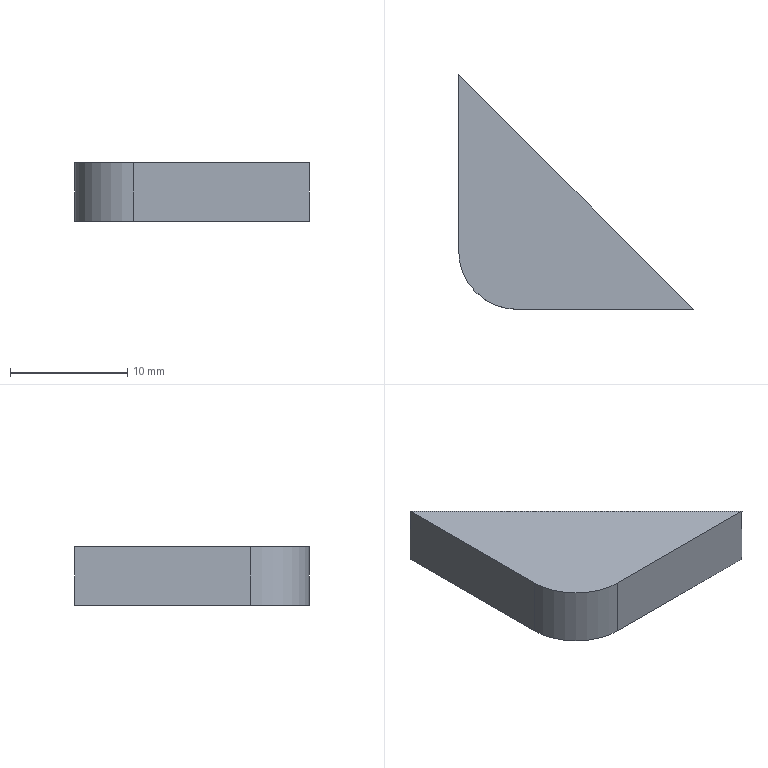Part | STEP file | Part8_5 | 1 solid | 6 faces | box 20 x 20 x 5 mm | volume 973.175 mm3 | plane 5 | cylinder 1 | commonest cylinder face diameters 10 x1
STEP:
#1=CARTESIAN_POINT('',(0.,0.,0.));
#2=DIRECTION('',(0.,0.,1.));
#3=DIRECTION('',(1.,0.,0.));
#4=AXIS2_PLACEMENT_3D('',#1,#2,#3);
#5=CARTESIAN_POINT('',(150.,24.941,-720.));
#6=VERTEX_POINT('',#5);
#7=CARTESIAN_POINT('',(130.,44.941,-720.));
#8=VERTEX_POINT('',#7);
#9=CARTESIAN_POINT('',(130.,44.941,-720.));
#10=DIRECTION('',(-0.7071,0.7071,0.));
#11=VECTOR('',#10,1.);
#12=LINE('',#9,#11);
#13=CARTESIAN_POINT('',(0.,0.,-720.));
#14=DIRECTION('',(0.,0.,-1.));
#15=DIRECTION('',(-1.,0.,0.));
#16=AXIS2_PLACEMENT_3D('',#13,#14,#15);
#17=PLANE('',#16);
#18=CARTESIAN_POINT('',(-130.,44.941));
#19=DIRECTION('',(0.7071,0.7071));
#20=VECTOR('',#19,1.);
#21=LINE('',#18,#20);
#22=(GEOMETRIC_REPRESENTATION_CONTEXT(2)PARAMETRIC_REPRESENTATION_CONTEXT()REPRESENTATION_CONTEXT('',''));
#23=DEFINITIONAL_REPRESENTATION('',(#21),#22);
#24=PCURVE('',#17,#23);
#25=CARTESIAN_POINT('',(130.,44.941,-685.));
#26=DIRECTION('',(0.7071,0.7071,0.));
#27=DIRECTION('',(-0.7071,0.7071,0.));
#28=AXIS2_PLACEMENT_3D('',#25,#26,#27);
#29=PLANE('',#28);
#30=CARTESIAN_POINT('',(0.,-35.));
#31=DIRECTION('',(1.,0.));
#32=VECTOR('',#31,1.);
#33=LINE('',#30,#32);
#34=(GEOMETRIC_REPRESENTATION_CONTEXT(2)PARAMETRIC_REPRESENTATION_CONTEXT()REPRESENTATION_CONTEXT('',''));
#35=DEFINITIONAL_REPRESENTATION('',(#33),#34);
#36=PCURVE('',#29,#35);
#37=SURFACE_CURVE('',#12,(#24,#36),.PCURVE_S1.);
#38=EDGE_CURVE('',#6,#8,#37,.T.);
#39=ORIENTED_EDGE('',*,*,#38,.F.);
#40=CARTESIAN_POINT('',(135.,24.941,-720.));
#41=VERTEX_POINT('',#40);
#42=CARTESIAN_POINT('',(135.,24.941,-720.));
#43=DIRECTION('',(-1.,0.,0.));
#44=VECTOR('',#43,1.);
#45=LINE('',#42,#44);
#46=CARTESIAN_POINT('',(-135.,24.941));
#47=DIRECTION('',(1.,0.));
#48=VECTOR('',#47,1.);
#49=LINE('',#46,#48);
#50=(GEOMETRIC_REPRESENTATION_CONTEXT(2)PARAMETRIC_REPRESENTATION_CONTEXT()REPRESENTATION_CONTEXT('',''));
#51=DEFINITIONAL_REPRESENTATION('',(#49),#50);
#52=PCURVE('',#17,#51);
#53=CARTESIAN_POINT('',(135.,24.941,-685.));
#54=DIRECTION('',(0.,1.,0.));
#55=DIRECTION('',(-1.,0.,0.));
#56=AXIS2_PLACEMENT_3D('',#53,#54,#55);
#57=PLANE('',#56);
#58=CARTESIAN_POINT('',(0.,-35.));
#59=DIRECTION('',(1.,0.));
#60=VECTOR('',#59,1.);
#61=LINE('',#58,#60);
#62=(GEOMETRIC_REPRESENTATION_CONTEXT(2)PARAMETRIC_REPRESENTATION_CONTEXT()REPRESENTATION_CONTEXT('',''));
#63=DEFINITIONAL_REPRESENTATION('',(#61),#62);
#64=PCURVE('',#57,#63);
#65=SURFACE_CURVE('',#45,(#52,#64),.PCURVE_S1.);
#66=EDGE_CURVE('',#6,#41,#65,.T.);
#67=ORIENTED_EDGE('',*,*,#66,.T.);
#68=CARTESIAN_POINT('',(130.,29.941,-720.));
#69=VERTEX_POINT('',#68);
#70=CARTESIAN_POINT('',(135.,29.941,-720.));
#71=DIRECTION('',(0.,0.,1.));
#72=DIRECTION('',(-1.,0.,0.));
#73=AXIS2_PLACEMENT_3D('',#70,#71,#72);
#74=CIRCLE('',#73,5.);
#75=CARTESIAN_POINT('',(-130.,29.941));
#76=CARTESIAN_POINT('',(-130.,21.281));
#77=CARTESIAN_POINT('',(-137.5,25.611));
#78=CARTESIAN_POINT('',(-145.,29.941));
#79=CARTESIAN_POINT('',(-137.5,34.271));
#80=CARTESIAN_POINT('',(-130.,38.602));
#81=CARTESIAN_POINT('',(-130.,29.941));
#82=(BOUNDED_CURVE()B_SPLINE_CURVE(2,(#75,#76,#77,#78,#79,#80,#81),.UNSPECIFIED.,.T.,.F.)B_SPLINE_CURVE_WITH_KNOTS((1,2,2,2,2,1),(-2.094,0.,2.094,4.189,6.283,8.378),.UNSPECIFIED.)CURVE()GEOMETRIC_REPRESENTATION_ITEM()RATIONAL_B_SPLINE_CURVE((1.,0.5,1.,0.5,1.,0.5,1.))REPRESENTATION_ITEM(''));
#83=(GEOMETRIC_REPRESENTATION_CONTEXT(2)PARAMETRIC_REPRESENTATION_CONTEXT()REPRESENTATION_CONTEXT('',''));
#84=DEFINITIONAL_REPRESENTATION('',(#82),#83);
#85=PCURVE('',#17,#84);
#86=CARTESIAN_POINT('',(135.,29.941,-717.5));
#87=DIRECTION('',(0.,0.,-1.));
#88=DIRECTION('',(-1.,0.,0.));
#89=AXIS2_PLACEMENT_3D('',#86,#87,#88);
#90=CYLINDRICAL_SURFACE('',#89,5.);
#91=CARTESIAN_POINT('',(6.283,2.5));
#92=DIRECTION('',(-1.,0.));
#93=VECTOR('',#92,1.);
#94=LINE('',#91,#93);
#95=(GEOMETRIC_REPRESENTATION_CONTEXT(2)PARAMETRIC_REPRESENTATION_CONTEXT()REPRESENTATION_CONTEXT('',''));
#96=DEFINITIONAL_REPRESENTATION('',(#94),#95);
#97=PCURVE('',#90,#96);
#98=SURFACE_CURVE('',#74,(#85,#97),.PCURVE_S1.);
#99=EDGE_CURVE('',#69,#41,#98,.T.);
#100=ORIENTED_EDGE('',*,*,#99,.F.);
#101=CARTESIAN_POINT('',(130.,29.941,-720.));
#102=DIRECTION('',(0.,-1.,0.));
#103=VECTOR('',#102,1.);
#104=LINE('',#101,#103);
#105=CARTESIAN_POINT('',(-130.,29.941));
#106=DIRECTION('',(0.,-1.));
#107=VECTOR('',#106,1.);
#108=LINE('',#105,#107);
#109=(GEOMETRIC_REPRESENTATION_CONTEXT(2)PARAMETRIC_REPRESENTATION_CONTEXT()REPRESENTATION_CONTEXT('',''));
#110=DEFINITIONAL_REPRESENTATION('',(#108),#109);
#111=PCURVE('',#17,#110);
#112=CARTESIAN_POINT('',(130.,29.941,-685.));
#113=DIRECTION('',(-1.,0.,0.));
#114=DIRECTION('',(0.,-1.,0.));
#115=AXIS2_PLACEMENT_3D('',#112,#113,#114);
#116=PLANE('',#115);
#117=CARTESIAN_POINT('',(0.,-35.));
#118=DIRECTION('',(1.,0.));
#119=VECTOR('',#118,1.);
#120=LINE('',#117,#119);
#121=(GEOMETRIC_REPRESENTATION_CONTEXT(2)PARAMETRIC_REPRESENTATION_CONTEXT()REPRESENTATION_CONTEXT('',''));
#122=DEFINITIONAL_REPRESENTATION('',(#120),#121);
#123=PCURVE('',#116,#122);
#124=SURFACE_CURVE('',#104,(#111,#123),.PCURVE_S1.);
#125=EDGE_CURVE('',#8,#69,#124,.T.);
#126=ORIENTED_EDGE('',*,*,#125,.F.);
#127=EDGE_LOOP('',(#39,#67,#100,#126));
#128=FACE_BOUND('',#127,.T.);
#129=ADVANCED_FACE('',(#128),#17,.T.);
#130=CARTESIAN_POINT('',(130.,29.941,-715.));
#131=VERTEX_POINT('',#130);
#132=CARTESIAN_POINT('',(130.,29.941,-685.));
#133=DIRECTION('',(0.,0.,1.));
#134=VECTOR('',#133,1.);
#135=LINE('',#132,#134);
#136=CARTESIAN_POINT('',(6.283,-32.5));
#137=DIRECTION('',(0.,-1.));
#138=VECTOR('',#137,1.);
#139=LINE('',#136,#138);
#140=(GEOMETRIC_REPRESENTATION_CONTEXT(2)PARAMETRIC_REPRESENTATION_CONTEXT()REPRESENTATION_CONTEXT('',''));
#141=DEFINITIONAL_REPRESENTATION('',(#139),#140);
#142=PCURVE('',#90,#141);
#143=CARTESIAN_POINT('',(0.,0.));
#144=DIRECTION('',(0.,1.));
#145=VECTOR('',#144,1.);
#146=LINE('',#143,#145);
#147=(GEOMETRIC_REPRESENTATION_CONTEXT(2)PARAMETRIC_REPRESENTATION_CONTEXT()REPRESENTATION_CONTEXT('',''));
#148=DEFINITIONAL_REPRESENTATION('',(#146),#147);
#149=PCURVE('',#116,#148);
#150=SURFACE_CURVE('',#135,(#142,#149),.PCURVE_S1.);
#151=EDGE_CURVE('',#69,#131,#150,.T.);
#152=ORIENTED_EDGE('',*,*,#151,.F.);
#153=ORIENTED_EDGE('',*,*,#99,.T.);
#154=CARTESIAN_POINT('',(135.,24.941,-715.));
#155=VERTEX_POINT('',#154);
#156=CARTESIAN_POINT('',(135.,24.941,-685.));
#157=DIRECTION('',(0.,0.,1.));
#158=VECTOR('',#157,1.);
#159=LINE('',#156,#158);
#160=CARTESIAN_POINT('',(4.712,-32.5));
#161=DIRECTION('',(0.,-1.));
#162=VECTOR('',#161,1.);
#163=LINE('',#160,#162);
#164=(GEOMETRIC_REPRESENTATION_CONTEXT(2)PARAMETRIC_REPRESENTATION_CONTEXT()REPRESENTATION_CONTEXT('',''));
#165=DEFINITIONAL_REPRESENTATION('',(#163),#164);
#166=PCURVE('',#90,#165);
#167=CARTESIAN_POINT('',(0.,0.));
#168=DIRECTION('',(0.,1.));
#169=VECTOR('',#168,1.);
#170=LINE('',#167,#169);
#171=(GEOMETRIC_REPRESENTATION_CONTEXT(2)PARAMETRIC_REPRESENTATION_CONTEXT()REPRESENTATION_CONTEXT('',''));
#172=DEFINITIONAL_REPRESENTATION('',(#170),#171);
#173=PCURVE('',#57,#172);
#174=SURFACE_CURVE('',#159,(#166,#173),.PCURVE_S1.);
#175=EDGE_CURVE('',#41,#155,#174,.T.);
#176=ORIENTED_EDGE('',*,*,#175,.T.);
#177=CARTESIAN_POINT('',(135.,29.941,-715.));
#178=DIRECTION('',(0.,0.,-1.));
#179=DIRECTION('',(-1.,0.,0.));
#180=AXIS2_PLACEMENT_3D('',#177,#178,#179);
#181=CIRCLE('',#180,5.);
#182=CARTESIAN_POINT('',(0.,-2.5));
#183=DIRECTION('',(1.,0.));
#184=VECTOR('',#183,1.);
#185=LINE('',#182,#184);
#186=(GEOMETRIC_REPRESENTATION_CONTEXT(2)PARAMETRIC_REPRESENTATION_CONTEXT()REPRESENTATION_CONTEXT('',''));
#187=DEFINITIONAL_REPRESENTATION('',(#185),#186);
#188=PCURVE('',#90,#187);
#189=CARTESIAN_POINT('',(0.,0.,-715.));
#190=DIRECTION('',(0.,0.,-1.));
#191=DIRECTION('',(-1.,0.,0.));
#192=AXIS2_PLACEMENT_3D('',#189,#190,#191);
#193=PLANE('',#192);
#194=CARTESIAN_POINT('',(-135.,29.941));
#195=DIRECTION('',(1.,0.));
#196=AXIS2_PLACEMENT_2D('',#194,#195);
#197=CIRCLE('',#196,5.);
#198=(GEOMETRIC_REPRESENTATION_CONTEXT(2)PARAMETRIC_REPRESENTATION_CONTEXT()REPRESENTATION_CONTEXT('',''));
#199=DEFINITIONAL_REPRESENTATION('',(#197),#198);
#200=PCURVE('',#193,#199);
#201=SURFACE_CURVE('',#181,(#188,#200),.PCURVE_S1.);
#202=EDGE_CURVE('',#155,#131,#201,.T.);
#203=ORIENTED_EDGE('',*,*,#202,.T.);
#204=EDGE_LOOP('',(#152,#153,#176,#203));
#205=FACE_BOUND('',#204,.T.);
#206=ADVANCED_FACE('',(#205),#90,.T.);
#207=CARTESIAN_POINT('',(130.,44.941,-715.));
#208=VERTEX_POINT('',#207);
#209=CARTESIAN_POINT('',(130.,44.941,-685.));
#210=DIRECTION('',(0.,0.,1.));
#211=VECTOR('',#210,1.);
#212=LINE('',#209,#211);
#213=CARTESIAN_POINT('',(-15.,0.));
#214=DIRECTION('',(0.,1.));
#215=VECTOR('',#214,1.);
#216=LINE('',#213,#215);
#217=(GEOMETRIC_REPRESENTATION_CONTEXT(2)PARAMETRIC_REPRESENTATION_CONTEXT()REPRESENTATION_CONTEXT('',''));
#218=DEFINITIONAL_REPRESENTATION('',(#216),#217);
#219=PCURVE('',#116,#218);
#220=CARTESIAN_POINT('',(0.,0.));
#221=DIRECTION('',(0.,1.));
#222=VECTOR('',#221,1.);
#223=LINE('',#220,#222);
#224=(GEOMETRIC_REPRESENTATION_CONTEXT(2)PARAMETRIC_REPRESENTATION_CONTEXT()REPRESENTATION_CONTEXT('',''));
#225=DEFINITIONAL_REPRESENTATION('',(#223),#224);
#226=PCURVE('',#29,#225);
#227=SURFACE_CURVE('',#212,(#219,#226),.PCURVE_S1.);
#228=EDGE_CURVE('',#8,#208,#227,.T.);
#229=ORIENTED_EDGE('',*,*,#228,.F.);
#230=ORIENTED_EDGE('',*,*,#125,.T.);
#231=ORIENTED_EDGE('',*,*,#151,.T.);
#232=CARTESIAN_POINT('',(130.,0.,-715.));
#233=DIRECTION('',(0.,1.,0.));
#234=VECTOR('',#233,1.);
#235=LINE('',#232,#234);
#236=CARTESIAN_POINT('',(29.941,-30.));
#237=DIRECTION('',(-1.,0.));
#238=VECTOR('',#237,1.);
#239=LINE('',#236,#238);
#240=(GEOMETRIC_REPRESENTATION_CONTEXT(2)PARAMETRIC_REPRESENTATION_CONTEXT()REPRESENTATION_CONTEXT('',''));
#241=DEFINITIONAL_REPRESENTATION('',(#239),#240);
#242=PCURVE('',#116,#241);
#243=CARTESIAN_POINT('',(-130.,0.));
#244=DIRECTION('',(0.,1.));
#245=VECTOR('',#244,1.);
#246=LINE('',#243,#245);
#247=(GEOMETRIC_REPRESENTATION_CONTEXT(2)PARAMETRIC_REPRESENTATION_CONTEXT()REPRESENTATION_CONTEXT('',''));
#248=DEFINITIONAL_REPRESENTATION('',(#246),#247);
#249=PCURVE('',#193,#248);
#250=SURFACE_CURVE('',#235,(#242,#249),.PCURVE_S1.);
#251=EDGE_CURVE('',#131,#208,#250,.T.);
#252=ORIENTED_EDGE('',*,*,#251,.T.);
#253=EDGE_LOOP('',(#229,#230,#231,#252));
#254=FACE_BOUND('',#253,.T.);
#255=ADVANCED_FACE('',(#254),#116,.T.);
#256=CARTESIAN_POINT('',(150.,24.941,-715.));
#257=VERTEX_POINT('',#256);
#258=CARTESIAN_POINT('',(150.,24.941,-685.));
#259=DIRECTION('',(0.,0.,-1.));
#260=VECTOR('',#259,1.);
#261=LINE('',#258,#260);
#262=CARTESIAN_POINT('',(-28.284,0.));
#263=DIRECTION('',(0.,-1.));
#264=VECTOR('',#263,1.);
#265=LINE('',#262,#264);
#266=(GEOMETRIC_REPRESENTATION_CONTEXT(2)PARAMETRIC_REPRESENTATION_CONTEXT()REPRESENTATION_CONTEXT('',''));
#267=DEFINITIONAL_REPRESENTATION('',(#265),#266);
#268=PCURVE('',#29,#267);
#269=CARTESIAN_POINT('',(-15.,0.));
#270=DIRECTION('',(0.,-1.));
#271=VECTOR('',#270,1.);
#272=LINE('',#269,#271);
#273=(GEOMETRIC_REPRESENTATION_CONTEXT(2)PARAMETRIC_REPRESENTATION_CONTEXT()REPRESENTATION_CONTEXT('',''));
#274=DEFINITIONAL_REPRESENTATION('',(#272),#273);
#275=PCURVE('',#57,#274);
#276=SURFACE_CURVE('',#261,(#268,#275),.PCURVE_S1.);
#277=EDGE_CURVE('',#257,#6,#276,.T.);
#278=ORIENTED_EDGE('',*,*,#277,.T.);
#279=ORIENTED_EDGE('',*,*,#38,.T.);
#280=ORIENTED_EDGE('',*,*,#228,.T.);
#281=CARTESIAN_POINT('',(130.,44.941,-715.));
#282=DIRECTION('',(0.7071,-0.7071,0.));
#283=VECTOR('',#282,1.);
#284=LINE('',#281,#283);
#285=CARTESIAN_POINT('',(0.,-30.));
#286=DIRECTION('',(-1.,0.));
#287=VECTOR('',#286,1.);
#288=LINE('',#285,#287);
#289=(GEOMETRIC_REPRESENTATION_CONTEXT(2)PARAMETRIC_REPRESENTATION_CONTEXT()REPRESENTATION_CONTEXT('',''));
#290=DEFINITIONAL_REPRESENTATION('',(#288),#289);
#291=PCURVE('',#29,#290);
#292=CARTESIAN_POINT('',(-130.,44.941));
#293=DIRECTION('',(-0.7071,-0.7071));
#294=VECTOR('',#293,1.);
#295=LINE('',#292,#294);
#296=(GEOMETRIC_REPRESENTATION_CONTEXT(2)PARAMETRIC_REPRESENTATION_CONTEXT()REPRESENTATION_CONTEXT('',''));
#297=DEFINITIONAL_REPRESENTATION('',(#295),#296);
#298=PCURVE('',#193,#297);
#299=SURFACE_CURVE('',#284,(#291,#298),.PCURVE_S1.);
#300=EDGE_CURVE('',#208,#257,#299,.T.);
#301=ORIENTED_EDGE('',*,*,#300,.T.);
#302=EDGE_LOOP('',(#278,#279,#280,#301));
#303=FACE_BOUND('',#302,.T.);
#304=ADVANCED_FACE('',(#303),#29,.T.);
#305=CARTESIAN_POINT('',(0.,24.941,-715.));
#306=DIRECTION('',(-1.,0.,0.));
#307=VECTOR('',#306,1.);
#308=LINE('',#305,#307);
#309=CARTESIAN_POINT('',(135.,-30.));
#310=DIRECTION('',(1.,0.));
#311=VECTOR('',#310,1.);
#312=LINE('',#309,#311);
#313=(GEOMETRIC_REPRESENTATION_CONTEXT(2)PARAMETRIC_REPRESENTATION_CONTEXT()REPRESENTATION_CONTEXT('',''));
#314=DEFINITIONAL_REPRESENTATION('',(#312),#313);
#315=PCURVE('',#57,#314);
#316=CARTESIAN_POINT('',(0.,24.941));
#317=DIRECTION('',(1.,0.));
#318=VECTOR('',#317,1.);
#319=LINE('',#316,#318);
#320=(GEOMETRIC_REPRESENTATION_CONTEXT(2)PARAMETRIC_REPRESENTATION_CONTEXT()REPRESENTATION_CONTEXT('',''));
#321=DEFINITIONAL_REPRESENTATION('',(#319),#320);
#322=PCURVE('',#193,#321);
#323=SURFACE_CURVE('',#308,(#315,#322),.PCURVE_S1.);
#324=EDGE_CURVE('',#257,#155,#323,.T.);
#325=ORIENTED_EDGE('',*,*,#324,.T.);
#326=ORIENTED_EDGE('',*,*,#175,.F.);
#327=ORIENTED_EDGE('',*,*,#66,.F.);
#328=ORIENTED_EDGE('',*,*,#277,.F.);
#329=EDGE_LOOP('',(#325,#326,#327,#328));
#330=FACE_BOUND('',#329,.T.);
#331=ADVANCED_FACE('',(#330),#57,.F.);
#332=ORIENTED_EDGE('',*,*,#300,.F.);
#333=ORIENTED_EDGE('',*,*,#251,.F.);
#334=ORIENTED_EDGE('',*,*,#202,.F.);
#335=ORIENTED_EDGE('',*,*,#324,.F.);
#336=EDGE_LOOP('',(#332,#333,#334,#335));
#337=FACE_BOUND('',#336,.T.);
#338=ADVANCED_FACE('',(#337),#193,.F.);
#339=CLOSED_SHELL('',(#129,#206,#255,#304,#331,#338));
#340=MANIFOLD_SOLID_BREP('',#339);
#341=(LENGTH_UNIT()NAMED_UNIT(*)SI_UNIT(.MILLI.,.METRE.));
#342=UNCERTAINTY_MEASURE_WITH_UNIT(LENGTH_MEASURE(0.0000001),#341,'','');
#343=(NAMED_UNIT(*)PLANE_ANGLE_UNIT()SI_UNIT($,.RADIAN.));
#344=(NAMED_UNIT(*)SI_UNIT($,.STERADIAN.)SOLID_ANGLE_UNIT());
#345=(GEOMETRIC_REPRESENTATION_CONTEXT(3)GLOBAL_UNCERTAINTY_ASSIGNED_CONTEXT((#342))GLOBAL_UNIT_ASSIGNED_CONTEXT((#341,#343,#344))REPRESENTATION_CONTEXT('',''));
#346=ADVANCED_BREP_SHAPE_REPRESENTATION('',(#4,#340),#345);